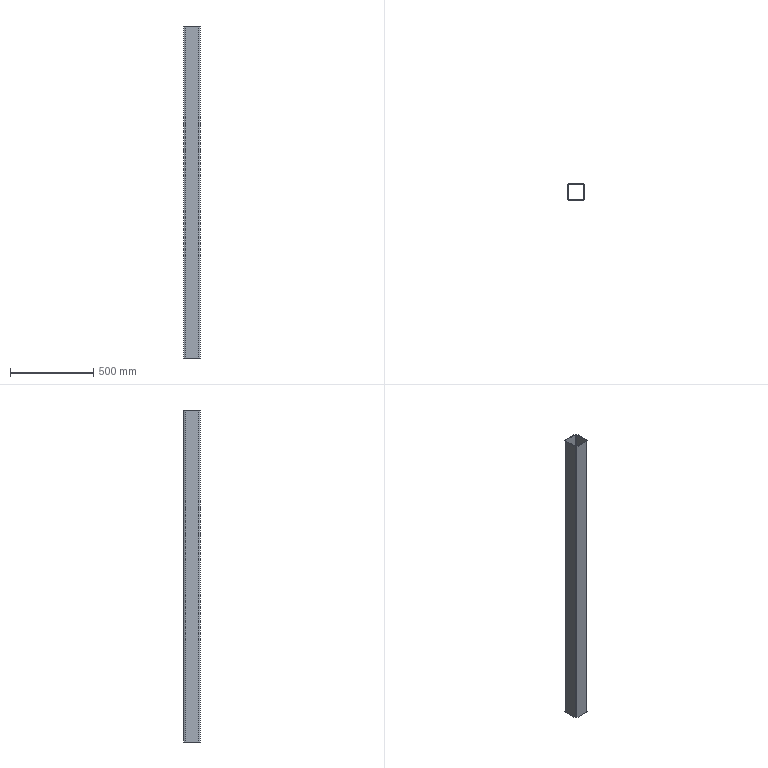Part | SolidWorks | features Extrusion 1, Fillet 1, HoleWzd 1, ICE 1, Shell 1 | 1 solid | 34 faces | box 100 x 100 x 2000 mm | volume 2980690 mm3 | cylinder 24 | plane 10 | commonest cylinder face diameters 6.8 x8 15 x8 8.8 x4 16.8 x4
STEP:
#1=CARTESIAN_POINT('',(-41.6,46.,1378.438));
#2=VERTEX_POINT('',#1);
#3=CARTESIAN_POINT('',(-35.,46.,1374.5));
#4=VERTEX_POINT('',#3);
#5=CARTESIAN_POINT('',(-35.,46.,1382.));
#6=DIRECTION('',(0.,-1.,0.));
#7=DIRECTION('',(0.,0.,-1.));
#8=AXIS2_PLACEMENT_3D('',#5,#6,#7);
#9=CIRCLE('',#8,7.5);
#10=EDGE_CURVE('',#2,#4,#9,.T.);
#11=ORIENTED_EDGE('',*,*,#10,.T.);
#12=CARTESIAN_POINT('',(-35.,50.,1374.5));
#13=VERTEX_POINT('',#12);
#14=CARTESIAN_POINT('',(-35.,40.,1374.5));
#15=DIRECTION('',(0.,1.,0.));
#16=VECTOR('',#15,1000.);
#17=LINE('',#14,#16);
#18=EDGE_CURVE('',#4,#13,#17,.T.);
#19=ORIENTED_EDGE('',*,*,#18,.T.);
#20=CARTESIAN_POINT('',(-41.6,50.,1378.438));
#21=VERTEX_POINT('',#20);
#22=CARTESIAN_POINT('',(-35.,50.,1382.));
#23=DIRECTION('',(0.,1.,0.));
#24=DIRECTION('',(0.,0.,1.));
#25=AXIS2_PLACEMENT_3D('',#22,#23,#24);
#26=CIRCLE('',#25,7.5);
#27=EDGE_CURVE('',#13,#21,#26,.T.);
#28=ORIENTED_EDGE('',*,*,#27,.T.);
#29=CARTESIAN_POINT('',(-41.6,50.,1385.562));
#30=VERTEX_POINT('',#29);
#31=CARTESIAN_POINT('',(-41.6,50.,1378.438));
#32=CARTESIAN_POINT('',(-41.897,50.,1378.987));
#33=CARTESIAN_POINT('',(-42.119,49.985,1379.562));
#34=CARTESIAN_POINT('',(-42.347,49.967,1380.459));
#35=CARTESIAN_POINT('',(-42.404,49.961,1380.767));
#36=CARTESIAN_POINT('',(-42.481,49.954,1381.383));
#37=CARTESIAN_POINT('',(-42.5,49.952,1381.691));
#38=CARTESIAN_POINT('',(-42.5,49.952,1382.307));
#39=CARTESIAN_POINT('',(-42.481,49.954,1382.614));
#40=CARTESIAN_POINT('',(-42.405,49.961,1383.229));
#41=CARTESIAN_POINT('',(-42.347,49.967,1383.537));
#42=CARTESIAN_POINT('',(-42.12,49.985,1384.438));
#43=CARTESIAN_POINT('',(-41.897,50.,1385.013));
#44=CARTESIAN_POINT('',(-41.6,50.,1385.562));
#45=B_SPLINE_CURVE_WITH_KNOTS('',3,(#31,#32,#33,#34,#35,#36,#37,#38,#39,#40,#41,#42,#43,#44),.UNSPECIFIED.,.F.,.F.,(4,2,2,2,2,2,4),(0.,0.001847,0.00277,0.003694,0.004617,0.00554,0.007387),.UNSPECIFIED.);
#46=EDGE_CURVE('',#21,#30,#45,.T.);
#47=ORIENTED_EDGE('',*,*,#46,.T.);
#48=CARTESIAN_POINT('',(-35.,50.,1389.5));
#49=VERTEX_POINT('',#48);
#50=CARTESIAN_POINT('',(-35.,50.,1382.));
#51=DIRECTION('',(0.,1.,0.));
#52=DIRECTION('',(0.,0.,1.));
#53=AXIS2_PLACEMENT_3D('',#50,#51,#52);
#54=CIRCLE('',#53,7.5);
#55=EDGE_CURVE('',#30,#49,#54,.T.);
#56=ORIENTED_EDGE('',*,*,#55,.T.);
#57=CARTESIAN_POINT('',(-35.,46.,1389.5));
#58=VERTEX_POINT('',#57);
#59=CARTESIAN_POINT('',(-35.,40.,1389.5));
#60=DIRECTION('',(0.,1.,0.));
#61=VECTOR('',#60,1000.);
#62=LINE('',#59,#61);
#63=EDGE_CURVE('',#58,#49,#62,.T.);
#64=ORIENTED_EDGE('',*,*,#63,.F.);
#65=CARTESIAN_POINT('',(-41.6,46.,1385.562));
#66=VERTEX_POINT('',#65);
#67=CARTESIAN_POINT('',(-35.,46.,1382.));
#68=DIRECTION('',(0.,-1.,0.));
#69=DIRECTION('',(0.,0.,-1.));
#70=AXIS2_PLACEMENT_3D('',#67,#68,#69);
#71=CIRCLE('',#70,7.5);
#72=EDGE_CURVE('',#58,#66,#71,.T.);
#73=ORIENTED_EDGE('',*,*,#72,.T.);
#74=CARTESIAN_POINT('',(-41.6,46.,1378.438));
#75=CARTESIAN_POINT('',(-41.897,46.,1378.988));
#76=CARTESIAN_POINT('',(-42.12,45.972,1379.563));
#77=CARTESIAN_POINT('',(-42.348,45.937,1380.466));
#78=CARTESIAN_POINT('',(-42.406,45.926,1380.774));
#79=CARTESIAN_POINT('',(-42.481,45.911,1381.387));
#80=CARTESIAN_POINT('',(-42.5,45.907,1381.695));
#81=CARTESIAN_POINT('',(-42.5,45.907,1382.311));
#82=CARTESIAN_POINT('',(-42.481,45.911,1382.619));
#83=CARTESIAN_POINT('',(-42.404,45.926,1383.238));
#84=CARTESIAN_POINT('',(-42.346,45.937,1383.543));
#85=CARTESIAN_POINT('',(-42.119,45.972,1384.439));
#86=CARTESIAN_POINT('',(-41.897,46.,1385.012));
#87=CARTESIAN_POINT('',(-41.6,46.,1385.562));
#88=B_SPLINE_CURVE_WITH_KNOTS('',3,(#74,#75,#76,#77,#78,#79,#80,#81,#82,#83,#84,#85,#86,#87),.UNSPECIFIED.,.F.,.F.,(4,2,2,2,2,2,4),(0.,0.001853,0.00278,0.003707,0.004633,0.00556,0.007413),.UNSPECIFIED.);
#89=EDGE_CURVE('',#2,#66,#88,.T.);
#90=ORIENTED_EDGE('',*,*,#89,.F.);
#91=EDGE_LOOP('',(#11,#19,#28,#47,#56,#64,#73,#90));
#92=FACE_OUTER_BOUND('',#91,.T.);
#93=CARTESIAN_POINT('',(-35.,40.,1382.));
#94=DIRECTION('',(0.,1.,0.));
#95=DIRECTION('',(0.,0.,1.));
#96=AXIS2_PLACEMENT_3D('',#93,#94,#95);
#97=CYLINDRICAL_SURFACE('',#96,7.5);
#98=ADVANCED_FACE('',(#92),#97,.F.);
#99=CARTESIAN_POINT('',(-41.6,46.,614.438));
#100=VERTEX_POINT('',#99);
#101=CARTESIAN_POINT('',(-35.,46.,610.5));
#102=VERTEX_POINT('',#101);
#103=CARTESIAN_POINT('',(-35.,46.,618.));
#104=DIRECTION('',(0.,-1.,0.));
#105=DIRECTION('',(0.,0.,-1.));
#106=AXIS2_PLACEMENT_3D('',#103,#104,#105);
#107=CIRCLE('',#106,7.5);
#108=EDGE_CURVE('',#100,#102,#107,.T.);
#109=ORIENTED_EDGE('',*,*,#108,.T.);
#110=CARTESIAN_POINT('',(-35.,50.,610.5));
#111=VERTEX_POINT('',#110);
#112=CARTESIAN_POINT('',(-35.,40.,610.5));
#113=DIRECTION('',(0.,1.,0.));
#114=VECTOR('',#113,1000.);
#115=LINE('',#112,#114);
#116=EDGE_CURVE('',#102,#111,#115,.T.);
#117=ORIENTED_EDGE('',*,*,#116,.T.);
#118=CARTESIAN_POINT('',(-41.6,50.,614.438));
#119=VERTEX_POINT('',#118);
#120=CARTESIAN_POINT('',(-35.,50.,618.));
#121=DIRECTION('',(0.,1.,0.));
#122=DIRECTION('',(0.,0.,1.));
#123=AXIS2_PLACEMENT_3D('',#120,#121,#122);
#124=CIRCLE('',#123,7.5);
#125=EDGE_CURVE('',#111,#119,#124,.T.);
#126=ORIENTED_EDGE('',*,*,#125,.T.);
#127=CARTESIAN_POINT('',(-41.6,50.,621.562));
#128=VERTEX_POINT('',#127);
#129=CARTESIAN_POINT('',(-41.6,50.,614.438));
#130=CARTESIAN_POINT('',(-41.897,50.,614.987));
#131=CARTESIAN_POINT('',(-42.119,49.985,615.562));
#132=CARTESIAN_POINT('',(-42.347,49.967,616.459));
#133=CARTESIAN_POINT('',(-42.404,49.961,616.767));
#134=CARTESIAN_POINT('',(-42.481,49.954,617.383));
#135=CARTESIAN_POINT('',(-42.5,49.952,617.691));
#136=CARTESIAN_POINT('',(-42.5,49.952,618.307));
#137=CARTESIAN_POINT('',(-42.481,49.954,618.614));
#138=CARTESIAN_POINT('',(-42.405,49.961,619.229));
#139=CARTESIAN_POINT('',(-42.347,49.967,619.537));
#140=CARTESIAN_POINT('',(-42.12,49.985,620.438));
#141=CARTESIAN_POINT('',(-41.897,50.,621.013));
#142=CARTESIAN_POINT('',(-41.6,50.,621.562));
#143=B_SPLINE_CURVE_WITH_KNOTS('',3,(#129,#130,#131,#132,#133,#134,#135,#136,#137,#138,#139,#140,#141,#142),.UNSPECIFIED.,.F.,.F.,(4,2,2,2,2,2,4),(0.,0.001847,0.00277,0.003694,0.004617,0.00554,0.007387),.UNSPECIFIED.);
#144=EDGE_CURVE('',#119,#128,#143,.T.);
#145=ORIENTED_EDGE('',*,*,#144,.T.);
#146=CARTESIAN_POINT('',(-35.,50.,625.5));
#147=VERTEX_POINT('',#146);
#148=CARTESIAN_POINT('',(-35.,50.,618.));
#149=DIRECTION('',(0.,1.,0.));
#150=DIRECTION('',(0.,0.,1.));
#151=AXIS2_PLACEMENT_3D('',#148,#149,#150);
#152=CIRCLE('',#151,7.5);
#153=EDGE_CURVE('',#128,#147,#152,.T.);
#154=ORIENTED_EDGE('',*,*,#153,.T.);
#155=CARTESIAN_POINT('',(-35.,46.,625.5));
#156=VERTEX_POINT('',#155);
#157=CARTESIAN_POINT('',(-35.,40.,625.5));
#158=DIRECTION('',(0.,1.,0.));
#159=VECTOR('',#158,1000.);
#160=LINE('',#157,#159);
#161=EDGE_CURVE('',#156,#147,#160,.T.);
#162=ORIENTED_EDGE('',*,*,#161,.F.);
#163=CARTESIAN_POINT('',(-41.6,46.,621.562));
#164=VERTEX_POINT('',#163);
#165=CARTESIAN_POINT('',(-35.,46.,618.));
#166=DIRECTION('',(0.,-1.,0.));
#167=DIRECTION('',(0.,0.,-1.));
#168=AXIS2_PLACEMENT_3D('',#165,#166,#167);
#169=CIRCLE('',#168,7.5);
#170=EDGE_CURVE('',#156,#164,#169,.T.);
#171=ORIENTED_EDGE('',*,*,#170,.T.);
#172=CARTESIAN_POINT('',(-41.6,46.,614.438));
#173=CARTESIAN_POINT('',(-41.897,46.,614.988));
#174=CARTESIAN_POINT('',(-42.12,45.972,615.563));
#175=CARTESIAN_POINT('',(-42.348,45.937,616.466));
#176=CARTESIAN_POINT('',(-42.406,45.926,616.774));
#177=CARTESIAN_POINT('',(-42.481,45.911,617.387));
#178=CARTESIAN_POINT('',(-42.5,45.907,617.695));
#179=CARTESIAN_POINT('',(-42.5,45.907,618.311));
#180=CARTESIAN_POINT('',(-42.481,45.911,618.619));
#181=CARTESIAN_POINT('',(-42.404,45.926,619.238));
#182=CARTESIAN_POINT('',(-42.346,45.937,619.543));
#183=CARTESIAN_POINT('',(-42.119,45.972,620.439));
#184=CARTESIAN_POINT('',(-41.897,46.,621.012));
#185=CARTESIAN_POINT('',(-41.6,46.,621.562));
#186=B_SPLINE_CURVE_WITH_KNOTS('',3,(#172,#173,#174,#175,#176,#177,#178,#179,#180,#181,#182,#183,#184,#185),.UNSPECIFIED.,.F.,.F.,(4,2,2,2,2,2,4),(0.,0.001853,0.00278,0.003707,0.004633,0.00556,0.007413),.UNSPECIFIED.);
#187=EDGE_CURVE('',#100,#164,#186,.T.);
#188=ORIENTED_EDGE('',*,*,#187,.F.);
#189=EDGE_LOOP('',(#109,#117,#126,#145,#154,#162,#171,#188));
#190=FACE_OUTER_BOUND('',#189,.T.);
#191=CARTESIAN_POINT('',(-35.,40.,618.));
#192=DIRECTION('',(0.,1.,0.));
#193=DIRECTION('',(0.,0.,1.));
#194=AXIS2_PLACEMENT_3D('',#191,#192,#193);
#195=CYLINDRICAL_SURFACE('',#194,7.5);
#196=ADVANCED_FACE('',(#190),#195,.F.);
#197=CARTESIAN_POINT('',(35.,46.,1389.5));
#198=VERTEX_POINT('',#197);
#199=CARTESIAN_POINT('',(35.,46.,1374.5));
#200=VERTEX_POINT('',#199);
#201=CARTESIAN_POINT('',(35.,46.,1382.));
#202=DIRECTION('',(0.,-1.,0.));
#203=DIRECTION('',(0.,0.,-1.));
#204=AXIS2_PLACEMENT_3D('',#201,#202,#203);
#205=CIRCLE('',#204,7.5);
#206=EDGE_CURVE('',#198,#200,#205,.T.);
#207=ORIENTED_EDGE('',*,*,#206,.T.);
#208=CARTESIAN_POINT('',(35.,50.,1374.5));
#209=VERTEX_POINT('',#208);
#210=CARTESIAN_POINT('',(35.,40.,1374.5));
#211=DIRECTION('',(0.,1.,0.));
#212=VECTOR('',#211,1000.);
#213=LINE('',#210,#212);
#214=EDGE_CURVE('',#200,#209,#213,.T.);
#215=ORIENTED_EDGE('',*,*,#214,.T.);
#216=CARTESIAN_POINT('',(35.,50.,1389.5));
#217=VERTEX_POINT('',#216);
#218=CARTESIAN_POINT('',(35.,50.,1382.));
#219=DIRECTION('',(0.,1.,0.));
#220=DIRECTION('',(0.,0.,1.));
#221=AXIS2_PLACEMENT_3D('',#218,#219,#220);
#222=CIRCLE('',#221,7.5);
#223=EDGE_CURVE('',#209,#217,#222,.T.);
#224=ORIENTED_EDGE('',*,*,#223,.T.);
#225=CARTESIAN_POINT('',(35.,40.,1389.5));
#226=DIRECTION('',(0.,1.,0.));
#227=VECTOR('',#226,1000.);
#228=LINE('',#225,#227);
#229=EDGE_CURVE('',#198,#217,#228,.T.);
#230=ORIENTED_EDGE('',*,*,#229,.F.);
#231=EDGE_LOOP('',(#207,#215,#224,#230));
#232=FACE_OUTER_BOUND('',#231,.T.);
#233=CARTESIAN_POINT('',(35.,40.,1382.));
#234=DIRECTION('',(0.,1.,0.));
#235=DIRECTION('',(0.,0.,1.));
#236=AXIS2_PLACEMENT_3D('',#233,#234,#235);
#237=CYLINDRICAL_SURFACE('',#236,7.5);
#238=ADVANCED_FACE('',(#232),#237,.F.);
#239=CARTESIAN_POINT('',(35.,46.,625.5));
#240=VERTEX_POINT('',#239);
#241=CARTESIAN_POINT('',(35.,46.,610.5));
#242=VERTEX_POINT('',#241);
#243=CARTESIAN_POINT('',(35.,46.,618.));
#244=DIRECTION('',(0.,-1.,0.));
#245=DIRECTION('',(0.,0.,-1.));
#246=AXIS2_PLACEMENT_3D('',#243,#244,#245);
#247=CIRCLE('',#246,7.5);
#248=EDGE_CURVE('',#240,#242,#247,.T.);
#249=ORIENTED_EDGE('',*,*,#248,.T.);
#250=CARTESIAN_POINT('',(35.,50.,610.5));
#251=VERTEX_POINT('',#250);
#252=CARTESIAN_POINT('',(35.,40.,610.5));
#253=DIRECTION('',(0.,1.,0.));
#254=VECTOR('',#253,1000.);
#255=LINE('',#252,#254);
#256=EDGE_CURVE('',#242,#251,#255,.T.);
#257=ORIENTED_EDGE('',*,*,#256,.T.);
#258=CARTESIAN_POINT('',(35.,50.,625.5));
#259=VERTEX_POINT('',#258);
#260=CARTESIAN_POINT('',(35.,50.,618.));
#261=DIRECTION('',(0.,1.,0.));
#262=DIRECTION('',(0.,0.,1.));
#263=AXIS2_PLACEMENT_3D('',#260,#261,#262);
#264=CIRCLE('',#263,7.5);
#265=EDGE_CURVE('',#251,#259,#264,.T.);
#266=ORIENTED_EDGE('',*,*,#265,.T.);
#267=CARTESIAN_POINT('',(35.,40.,625.5));
#268=DIRECTION('',(0.,1.,0.));
#269=VECTOR('',#268,1000.);
#270=LINE('',#267,#269);
#271=EDGE_CURVE('',#240,#259,#270,.T.);
#272=ORIENTED_EDGE('',*,*,#271,.F.);
#273=EDGE_LOOP('',(#249,#257,#266,#272));
#274=FACE_OUTER_BOUND('',#273,.T.);
#275=CARTESIAN_POINT('',(35.,40.,618.));
#276=DIRECTION('',(0.,1.,0.));
#277=DIRECTION('',(0.,0.,1.));
#278=AXIS2_PLACEMENT_3D('',#275,#276,#277);
#279=CYLINDRICAL_SURFACE('',#278,7.5);
#280=ADVANCED_FACE('',(#274),#279,.F.);
#281=CARTESIAN_POINT('',(-35.,46.,393.4));
#282=VERTEX_POINT('',#281);
#283=CARTESIAN_POINT('',(-35.,46.,386.6));
#284=VERTEX_POINT('',#283);
#285=CARTESIAN_POINT('',(-35.,46.,390.));
#286=DIRECTION('',(0.,-1.,0.));
#287=DIRECTION('',(0.,0.,-1.));
#288=AXIS2_PLACEMENT_3D('',#285,#286,#287);
#289=CIRCLE('',#288,3.4);
#290=EDGE_CURVE('',#282,#284,#289,.T.);
#291=ORIENTED_EDGE('',*,*,#290,.T.);
#292=CARTESIAN_POINT('',(-35.,50.,386.6));
#293=VERTEX_POINT('',#292);
#294=CARTESIAN_POINT('',(-35.,50.,386.6));
#295=DIRECTION('',(0.,1.,0.));
#296=VECTOR('',#295,1000.);
#297=LINE('',#294,#296);
#298=EDGE_CURVE('',#284,#293,#297,.T.);
#299=ORIENTED_EDGE('',*,*,#298,.T.);
#300=CARTESIAN_POINT('',(-35.,50.,393.4));
#301=VERTEX_POINT('',#300);
#302=CARTESIAN_POINT('',(-35.,50.,390.));
#303=DIRECTION('',(0.,1.,0.));
#304=DIRECTION('',(0.,0.,1.));
#305=AXIS2_PLACEMENT_3D('',#302,#303,#304);
#306=CIRCLE('',#305,3.4);
#307=EDGE_CURVE('',#293,#301,#306,.T.);
#308=ORIENTED_EDGE('',*,*,#307,.T.);
#309=CARTESIAN_POINT('',(-35.,50.,393.4));
#310=DIRECTION('',(0.,1.,0.));
#311=VECTOR('',#310,1000.);
#312=LINE('',#309,#311);
#313=EDGE_CURVE('',#282,#301,#312,.T.);
#314=ORIENTED_EDGE('',*,*,#313,.F.);
#315=EDGE_LOOP('',(#291,#299,#308,#314));
#316=FACE_OUTER_BOUND('',#315,.T.);
#317=CARTESIAN_POINT('',(-35.,50.,390.));
#318=DIRECTION('',(0.,1.,0.));
#319=DIRECTION('',(0.,0.,1.));
#320=AXIS2_PLACEMENT_3D('',#317,#318,#319);
#321=CYLINDRICAL_SURFACE('',#320,3.4);
#322=ADVANCED_FACE('',(#316),#321,.F.);
#323=CARTESIAN_POINT('',(35.,46.,393.4));
#324=VERTEX_POINT('',#323);
#325=CARTESIAN_POINT('',(35.,46.,386.6));
#326=VERTEX_POINT('',#325);
#327=CARTESIAN_POINT('',(35.,46.,390.));
#328=DIRECTION('',(0.,-1.,0.));
#329=DIRECTION('',(0.,0.,-1.));
#330=AXIS2_PLACEMENT_3D('',#327,#328,#329);
#331=CIRCLE('',#330,3.4);
#332=EDGE_CURVE('',#324,#326,#331,.T.);
#333=ORIENTED_EDGE('',*,*,#332,.T.);
#334=CARTESIAN_POINT('',(35.,50.,386.6));
#335=VERTEX_POINT('',#334);
#336=CARTESIAN_POINT('',(35.,50.,386.6));
#337=DIRECTION('',(0.,1.,0.));
#338=VECTOR('',#337,1000.);
#339=LINE('',#336,#338);
#340=EDGE_CURVE('',#326,#335,#339,.T.);
#341=ORIENTED_EDGE('',*,*,#340,.T.);
#342=CARTESIAN_POINT('',(35.,50.,393.4));
#343=VERTEX_POINT('',#342);
#344=CARTESIAN_POINT('',(35.,50.,390.));
#345=DIRECTION('',(0.,1.,0.));
#346=DIRECTION('',(0.,0.,1.));
#347=AXIS2_PLACEMENT_3D('',#344,#345,#346);
#348=CIRCLE('',#347,3.4);
#349=EDGE_CURVE('',#335,#343,#348,.T.);
#350=ORIENTED_EDGE('',*,*,#349,.T.);
#351=CARTESIAN_POINT('',(35.,50.,393.4));
#352=DIRECTION('',(0.,1.,0.));
#353=VECTOR('',#352,1000.);
#354=LINE('',#351,#353);
#355=EDGE_CURVE('',#324,#343,#354,.T.);
#356=ORIENTED_EDGE('',*,*,#355,.F.);
#357=EDGE_LOOP('',(#333,#341,#350,#356));
#358=FACE_OUTER_BOUND('',#357,.T.);
#359=CARTESIAN_POINT('',(35.,50.,390.));
#360=DIRECTION('',(0.,1.,0.));
#361=DIRECTION('',(0.,0.,1.));
#362=AXIS2_PLACEMENT_3D('',#359,#360,#361);
#363=CYLINDRICAL_SURFACE('',#362,3.4);
#364=ADVANCED_FACE('',(#358),#363,.F.);
#365=CARTESIAN_POINT('',(35.,46.,483.4));
#366=VERTEX_POINT('',#365);
#367=CARTESIAN_POINT('',(35.,46.,476.6));
#368=VERTEX_POINT('',#367);
#369=CARTESIAN_POINT('',(35.,46.,480.));
#370=DIRECTION('',(0.,-1.,0.));
#371=DIRECTION('',(0.,0.,-1.));
#372=AXIS2_PLACEMENT_3D('',#369,#370,#371);
#373=CIRCLE('',#372,3.4);
#374=EDGE_CURVE('',#366,#368,#373,.T.);
#375=ORIENTED_EDGE('',*,*,#374,.T.);
#376=CARTESIAN_POINT('',(35.,50.,476.6));
#377=VERTEX_POINT('',#376);
#378=CARTESIAN_POINT('',(35.,50.,476.6));
#379=DIRECTION('',(0.,1.,0.));
#380=VECTOR('',#379,1000.);
#381=LINE('',#378,#380);
#382=EDGE_CURVE('',#368,#377,#381,.T.);
#383=ORIENTED_EDGE('',*,*,#382,.T.);
#384=CARTESIAN_POINT('',(35.,50.,483.4));
#385=VERTEX_POINT('',#384);
#386=CARTESIAN_POINT('',(35.,50.,480.));
#387=DIRECTION('',(0.,1.,0.));
#388=DIRECTION('',(0.,0.,1.));
#389=AXIS2_PLACEMENT_3D('',#386,#387,#388);
#390=CIRCLE('',#389,3.4);
#391=EDGE_CURVE('',#377,#385,#390,.T.);
#392=ORIENTED_EDGE('',*,*,#391,.T.);
#393=CARTESIAN_POINT('',(35.,50.,483.4));
#394=DIRECTION('',(0.,1.,0.));
#395=VECTOR('',#394,1000.);
#396=LINE('',#393,#395);
#397=EDGE_CURVE('',#366,#385,#396,.T.);
#398=ORIENTED_EDGE('',*,*,#397,.F.);
#399=EDGE_LOOP('',(#375,#383,#392,#398));
#400=FACE_OUTER_BOUND('',#399,.T.);
#401=CARTESIAN_POINT('',(35.,50.,480.));
#402=DIRECTION('',(0.,1.,0.));
#403=DIRECTION('',(0.,0.,1.));
#404=AXIS2_PLACEMENT_3D('',#401,#402,#403);
#405=CYLINDRICAL_SURFACE('',#404,3.4);
#406=ADVANCED_FACE('',(#400),#405,.F.);
#407=CARTESIAN_POINT('',(-35.,46.,483.4));
#408=VERTEX_POINT('',#407);
#409=CARTESIAN_POINT('',(-35.,46.,476.6));
#410=VERTEX_POINT('',#409);
#411=CARTESIAN_POINT('',(-35.,46.,480.));
#412=DIRECTION('',(0.,-1.,0.));
#413=DIRECTION('',(0.,0.,-1.));
#414=AXIS2_PLACEMENT_3D('',#411,#412,#413);
#415=CIRCLE('',#414,3.4);
#416=EDGE_CURVE('',#408,#410,#415,.T.);
#417=ORIENTED_EDGE('',*,*,#416,.T.);
#418=CARTESIAN_POINT('',(-35.,50.,476.6));
#419=VERTEX_POINT('',#418);
#420=CARTESIAN_POINT('',(-35.,50.,476.6));
#421=DIRECTION('',(0.,1.,0.));
#422=VECTOR('',#421,1000.);
#423=LINE('',#420,#422);
#424=EDGE_CURVE('',#410,#419,#423,.T.);
#425=ORIENTED_EDGE('',*,*,#424,.T.);
#426=CARTESIAN_POINT('',(-35.,50.,483.4));
#427=VERTEX_POINT('',#426);
#428=CARTESIAN_POINT('',(-35.,50.,480.));
#429=DIRECTION('',(0.,1.,0.));
#430=DIRECTION('',(0.,0.,1.));
#431=AXIS2_PLACEMENT_3D('',#428,#429,#430);
#432=CIRCLE('',#431,3.4);
#433=EDGE_CURVE('',#419,#427,#432,.T.);
#434=ORIENTED_EDGE('',*,*,#433,.T.);
#435=CARTESIAN_POINT('',(-35.,50.,483.4));
#436=DIRECTION('',(0.,1.,0.));
#437=VECTOR('',#436,1000.);
#438=LINE('',#435,#437);
#439=EDGE_CURVE('',#408,#427,#438,.T.);
#440=ORIENTED_EDGE('',*,*,#439,.F.);
#441=EDGE_LOOP('',(#417,#425,#434,#440));
#442=FACE_OUTER_BOUND('',#441,.T.);
#443=CARTESIAN_POINT('',(-35.,50.,480.));
#444=DIRECTION('',(0.,1.,0.));
#445=DIRECTION('',(0.,0.,1.));
#446=AXIS2_PLACEMENT_3D('',#443,#444,#445);
#447=CYLINDRICAL_SURFACE('',#446,3.4);
#448=ADVANCED_FACE('',(#442),#447,.F.);
#449=CARTESIAN_POINT('',(50.,-41.6,0.));
#450=VERTEX_POINT('',#449);
#451=CARTESIAN_POINT('',(50.,41.6,0.));
#452=VERTEX_POINT('',#451);
#453=CARTESIAN_POINT('',(50.,50.,0.));
#454=DIRECTION('',(0.,1.,0.));
#455=VECTOR('',#454,1000.);
#456=LINE('',#453,#455);
#457=EDGE_CURVE('',#450,#452,#456,.T.);
#458=ORIENTED_EDGE('',*,*,#457,.F.);
#459=CARTESIAN_POINT('',(41.6,-50.,0.));
#460=VERTEX_POINT('',#459);
#461=CARTESIAN_POINT('',(41.6,-41.6,0.));
#462=DIRECTION('',(0.,0.,-1.));
#463=DIRECTION('',(-1.,0.,0.));
#464=AXIS2_PLACEMENT_3D('',#461,#462,#463);
#465=CIRCLE('',#464,8.4);
#466=EDGE_CURVE('',#450,#460,#465,.T.);
#467=ORIENTED_EDGE('',*,*,#466,.T.);
#468=CARTESIAN_POINT('',(-41.6,-50.,0.));
#469=VERTEX_POINT('',#468);
#470=CARTESIAN_POINT('',(50.,-50.,0.));
#471=DIRECTION('',(1.,0.,0.));
#472=VECTOR('',#471,1000.);
#473=LINE('',#470,#472);
#474=EDGE_CURVE('',#469,#460,#473,.T.);
#475=ORIENTED_EDGE('',*,*,#474,.F.);
#476=CARTESIAN_POINT('',(-50.,-41.6,0.));
#477=VERTEX_POINT('',#476);
#478=CARTESIAN_POINT('',(-41.6,-41.6,0.));
#479=DIRECTION('',(0.,0.,-1.));
#480=DIRECTION('',(-1.,0.,0.));
#481=AXIS2_PLACEMENT_3D('',#478,#479,#480);
#482=CIRCLE('',#481,8.4);
#483=EDGE_CURVE('',#469,#477,#482,.T.);
#484=ORIENTED_EDGE('',*,*,#483,.T.);
#485=CARTESIAN_POINT('',(-50.,41.6,0.));
#486=VERTEX_POINT('',#485);
#487=CARTESIAN_POINT('',(-50.,50.,0.));
#488=DIRECTION('',(0.,-1.,0.));
#489=VECTOR('',#488,1000.);
#490=LINE('',#487,#489);
#491=EDGE_CURVE('',#486,#477,#490,.T.);
#492=ORIENTED_EDGE('',*,*,#491,.F.);
#493=CARTESIAN_POINT('',(-41.6,50.,0.));
#494=VERTEX_POINT('',#493);
#495=CARTESIAN_POINT('',(-41.6,41.6,0.));
#496=DIRECTION('',(0.,0.,-1.));
#497=DIRECTION('',(-1.,0.,0.));
#498=AXIS2_PLACEMENT_3D('',#495,#496,#497);
#499=CIRCLE('',#498,8.4);
#500=EDGE_CURVE('',#486,#494,#499,.T.);
#501=ORIENTED_EDGE('',*,*,#500,.T.);
#502=CARTESIAN_POINT('',(41.6,50.,0.));
#503=VERTEX_POINT('',#502);
#504=CARTESIAN_POINT('',(50.,50.,0.));
#505=DIRECTION('',(-1.,0.,0.));
#506=VECTOR('',#505,1000.);
#507=LINE('',#504,#506);
#508=EDGE_CURVE('',#503,#494,#507,.T.);
#509=ORIENTED_EDGE('',*,*,#508,.F.);
#510=CARTESIAN_POINT('',(41.6,41.6,0.));
#511=DIRECTION('',(0.,0.,-1.));
#512=DIRECTION('',(-1.,0.,0.));
#513=AXIS2_PLACEMENT_3D('',#510,#511,#512);
#514=CIRCLE('',#513,8.4);
#515=EDGE_CURVE('',#503,#452,#514,.T.);
#516=ORIENTED_EDGE('',*,*,#515,.T.);
#517=EDGE_LOOP('',(#458,#467,#475,#484,#492,#501,#509,#516));
#518=FACE_OUTER_BOUND('',#517,.T.);
#519=CARTESIAN_POINT('',(46.,-41.6,0.));
#520=VERTEX_POINT('',#519);
#521=CARTESIAN_POINT('',(41.6,-46.,0.));
#522=VERTEX_POINT('',#521);
#523=CARTESIAN_POINT('',(41.6,-41.6,0.));
#524=DIRECTION('',(0.,0.,-1.));
#525=DIRECTION('',(-1.,0.,0.));
#526=AXIS2_PLACEMENT_3D('',#523,#524,#525);
#527=CIRCLE('',#526,4.4);
#528=EDGE_CURVE('',#520,#522,#527,.T.);
#529=ORIENTED_EDGE('',*,*,#528,.F.);
#530=CARTESIAN_POINT('',(46.,41.6,0.));
#531=VERTEX_POINT('',#530);
#532=CARTESIAN_POINT('',(46.,0.,0.));
#533=DIRECTION('',(0.,1.,0.));
#534=VECTOR('',#533,1000.);
#535=LINE('',#532,#534);
#536=EDGE_CURVE('',#520,#531,#535,.T.);
#537=ORIENTED_EDGE('',*,*,#536,.T.);
#538=CARTESIAN_POINT('',(41.6,46.,0.));
#539=VERTEX_POINT('',#538);
#540=CARTESIAN_POINT('',(41.6,41.6,0.));
#541=DIRECTION('',(0.,0.,-1.));
#542=DIRECTION('',(-1.,0.,0.));
#543=AXIS2_PLACEMENT_3D('',#540,#541,#542);
#544=CIRCLE('',#543,4.4);
#545=EDGE_CURVE('',#539,#531,#544,.T.);
#546=ORIENTED_EDGE('',*,*,#545,.F.);
#547=CARTESIAN_POINT('',(-41.6,46.,0.));
#548=VERTEX_POINT('',#547);
#549=CARTESIAN_POINT('',(0.,46.,0.));
#550=DIRECTION('',(-1.,0.,0.));
#551=VECTOR('',#550,1000.);
#552=LINE('',#549,#551);
#553=EDGE_CURVE('',#539,#548,#552,.T.);
#554=ORIENTED_EDGE('',*,*,#553,.T.);
#555=CARTESIAN_POINT('',(-46.,41.6,0.));
#556=VERTEX_POINT('',#555);
#557=CARTESIAN_POINT('',(-41.6,41.6,0.));
#558=DIRECTION('',(0.,0.,-1.));
#559=DIRECTION('',(-1.,0.,0.));
#560=AXIS2_PLACEMENT_3D('',#557,#558,#559);
#561=CIRCLE('',#560,4.4);
#562=EDGE_CURVE('',#556,#548,#561,.T.);
#563=ORIENTED_EDGE('',*,*,#562,.F.);
#564=CARTESIAN_POINT('',(-46.,-41.6,0.));
#565=VERTEX_POINT('',#564);
#566=CARTESIAN_POINT('',(-46.,0.,0.));
#567=DIRECTION('',(0.,-1.,0.));
#568=VECTOR('',#567,1000.);
#569=LINE('',#566,#568);
#570=EDGE_CURVE('',#556,#565,#569,.T.);
#571=ORIENTED_EDGE('',*,*,#570,.T.);
#572=CARTESIAN_POINT('',(-41.6,-46.,0.));
#573=VERTEX_POINT('',#572);
#574=CARTESIAN_POINT('',(-41.6,-41.6,0.));
#575=DIRECTION('',(0.,0.,-1.));
#576=DIRECTION('',(-1.,0.,0.));
#577=AXIS2_PLACEMENT_3D('',#574,#575,#576);
#578=CIRCLE('',#577,4.4);
#579=EDGE_CURVE('',#573,#565,#578,.T.);
#580=ORIENTED_EDGE('',*,*,#579,.F.);
#581=CARTESIAN_POINT('',(0.,-46.,0.));
#582=DIRECTION('',(1.,0.,0.));
#583=VECTOR('',#582,1000.);
#584=LINE('',#581,#583);
#585=EDGE_CURVE('',#573,#522,#584,.T.);
#586=ORIENTED_EDGE('',*,*,#585,.T.);
#587=EDGE_LOOP('',(#529,#537,#546,#554,#563,#571,#580,#586));
#588=FACE_BOUND('',#587,.T.);
#589=CARTESIAN_POINT('',(0.,0.,0.));
#590=DIRECTION('',(0.,0.,-1.));
#591=DIRECTION('',(-1.,0.,0.));
#592=AXIS2_PLACEMENT_3D('',#589,#590,#591);
#593=PLANE('',#592);
#594=ADVANCED_FACE('',(#518,#588),#593,.T.);
#595=ORIENTED_EDGE('',*,*,#491,.T.);
#596=CARTESIAN_POINT('',(-50.,-41.6,2000.));
#597=VERTEX_POINT('',#596);
#598=CARTESIAN_POINT('',(-50.,-41.6,2000.));
#599=DIRECTION('',(0.,0.,1.));
#600=VECTOR('',#599,1000.);
#601=LINE('',#598,#600);
#602=EDGE_CURVE('',#477,#597,#601,.T.);
#603=ORIENTED_EDGE('',*,*,#602,.T.);
#604=CARTESIAN_POINT('',(-50.,41.6,2000.));
#605=VERTEX_POINT('',#604);
#606=CARTESIAN_POINT('',(-50.,50.,2000.));
#607=DIRECTION('',(0.,-1.,0.));
#608=VECTOR('',#607,1000.);
#609=LINE('',#606,#608);
#610=EDGE_CURVE('',#605,#597,#609,.T.);
#611=ORIENTED_EDGE('',*,*,#610,.F.);
#612=CARTESIAN_POINT('',(-50.,41.6,2000.));
#613=DIRECTION('',(0.,0.,-1.));
#614=VECTOR('',#613,1000.);
#615=LINE('',#612,#614);
#616=EDGE_CURVE('',#605,#486,#615,.T.);
#617=ORIENTED_EDGE('',*,*,#616,.T.);
#618=EDGE_LOOP('',(#595,#603,#611,#617));
#619=FACE_OUTER_BOUND('',#618,.T.);
#620=CARTESIAN_POINT('',(-50.,50.,2000.));
#621=DIRECTION('',(1.,0.,0.));
#622=DIRECTION('',(0.,1.,0.));
#623=AXIS2_PLACEMENT_3D('',#620,#621,#622);
#624=PLANE('',#623);
#625=ADVANCED_FACE('',(#619),#624,.F.);
#626=ORIENTED_EDGE('',*,*,#474,.T.);
#627=CARTESIAN_POINT('',(41.6,-50.,2000.));
#628=VERTEX_POINT('',#627);
#629=CARTESIAN_POINT('',(41.6,-50.,2000.));
#630=DIRECTION('',(0.,0.,1.));
#631=VECTOR('',#630,1000.);
#632=LINE('',#629,#631);
#633=EDGE_CURVE('',#460,#628,#632,.T.);
#634=ORIENTED_EDGE('',*,*,#633,.T.);
#635=CARTESIAN_POINT('',(-41.6,-50.,2000.));
#636=VERTEX_POINT('',#635);
#637=CARTESIAN_POINT('',(50.,-50.,2000.));
#638=DIRECTION('',(1.,0.,0.));
#639=VECTOR('',#638,1000.);
#640=LINE('',#637,#639);
#641=EDGE_CURVE('',#636,#628,#640,.T.);
#642=ORIENTED_EDGE('',*,*,#641,.F.);
#643=CARTESIAN_POINT('',(-41.6,-50.,2000.));
#644=DIRECTION('',(0.,0.,-1.));
#645=VECTOR('',#644,1000.);
#646=LINE('',#643,#645);
#647=EDGE_CURVE('',#636,#469,#646,.T.);
#648=ORIENTED_EDGE('',*,*,#647,.T.);
#649=EDGE_LOOP('',(#626,#634,#642,#648));
#650=FACE_OUTER_BOUND('',#649,.T.);
#651=CARTESIAN_POINT('',(50.,-50.,2000.));
#652=DIRECTION('',(0.,1.,0.));
#653=DIRECTION('',(0.,0.,1.));
#654=AXIS2_PLACEMENT_3D('',#651,#652,#653);
#655=PLANE('',#654);
#656=ADVANCED_FACE('',(#650),#655,.F.);
#657=CARTESIAN_POINT('',(50.,-41.6,2000.));
#658=VERTEX_POINT('',#657);
#659=CARTESIAN_POINT('',(50.,41.6,2000.));
#660=VERTEX_POINT('',#659);
#661=CARTESIAN_POINT('',(50.,50.,2000.));
#662=DIRECTION('',(0.,1.,0.));
#663=VECTOR('',#662,1000.);
#664=LINE('',#661,#663);
#665=EDGE_CURVE('',#658,#660,#664,.T.);
#666=ORIENTED_EDGE('',*,*,#665,.F.);
#667=CARTESIAN_POINT('',(50.,-41.6,2000.));
#668=DIRECTION('',(0.,0.,-1.));
#669=VECTOR('',#668,1000.);
#670=LINE('',#667,#669);
#671=EDGE_CURVE('',#658,#450,#670,.T.);
#672=ORIENTED_EDGE('',*,*,#671,.T.);
#673=ORIENTED_EDGE('',*,*,#457,.T.);
#674=CARTESIAN_POINT('',(50.,41.6,2000.));
#675=DIRECTION('',(0.,0.,1.));
#676=VECTOR('',#675,1000.);
#677=LINE('',#674,#676);
#678=EDGE_CURVE('',#452,#660,#677,.T.);
#679=ORIENTED_EDGE('',*,*,#678,.T.);
#680=EDGE_LOOP('',(#666,#672,#673,#679));
#681=FACE_OUTER_BOUND('',#680,.T.);
#682=CARTESIAN_POINT('',(50.,50.,2000.));
#683=DIRECTION('',(-1.,0.,0.));
#684=DIRECTION('',(0.,-1.,0.));
#685=AXIS2_PLACEMENT_3D('',#682,#683,#684);
#686=PLANE('',#685);
#687=ADVANCED_FACE('',(#681),#686,.F.);
#688=CARTESIAN_POINT('',(-35.,50.,390.));
#689=DIRECTION('',(0.,1.,0.));
#690=DIRECTION('',(0.,0.,1.));
#691=AXIS2_PLACEMENT_3D('',#688,#689,#690);
#692=CIRCLE('',#691,3.4);
#693=EDGE_CURVE('',#301,#293,#692,.T.);
#694=ORIENTED_EDGE('',*,*,#693,.F.);
#695=ORIENTED_EDGE('',*,*,#307,.F.);
#696=EDGE_LOOP('',(#694,#695));
#697=FACE_BOUND('',#696,.T.);
#698=CARTESIAN_POINT('',(35.,50.,390.));
#699=DIRECTION('',(0.,1.,0.));
#700=DIRECTION('',(0.,0.,1.));
#701=AXIS2_PLACEMENT_3D('',#698,#699,#700);
#702=CIRCLE('',#701,3.4);
#703=EDGE_CURVE('',#343,#335,#702,.T.);
#704=ORIENTED_EDGE('',*,*,#703,.F.);
#705=ORIENTED_EDGE('',*,*,#349,.F.);
#706=EDGE_LOOP('',(#704,#705));
#707=FACE_BOUND('',#706,.T.);
#708=CARTESIAN_POINT('',(35.,50.,480.));
#709=DIRECTION('',(0.,1.,0.));
#710=DIRECTION('',(0.,0.,1.));
#711=AXIS2_PLACEMENT_3D('',#708,#709,#710);
#712=CIRCLE('',#711,3.4);
#713=EDGE_CURVE('',#385,#377,#712,.T.);
#714=ORIENTED_EDGE('',*,*,#713,.F.);
#715=ORIENTED_EDGE('',*,*,#391,.F.);
#716=EDGE_LOOP('',(#714,#715));
#717=FACE_BOUND('',#716,.T.);
#718=CARTESIAN_POINT('',(-35.,50.,480.));
#719=DIRECTION('',(0.,1.,0.));
#720=DIRECTION('',(0.,0.,1.));
#721=AXIS2_PLACEMENT_3D('',#718,#719,#720);
#722=CIRCLE('',#721,3.4);
#723=EDGE_CURVE('',#427,#419,#722,.T.);
#724=ORIENTED_EDGE('',*,*,#723,.F.);
#725=ORIENTED_EDGE('',*,*,#433,.F.);
#726=EDGE_LOOP('',(#724,#725));
#727=FACE_BOUND('',#726,.T.);
#728=CARTESIAN_POINT('',(-41.6,50.,2000.));
#729=DIRECTION('',(0.,0.,1.));
#730=VECTOR('',#729,1000.);
#731=LINE('',#728,#730);
#732=EDGE_CURVE('',#128,#21,#731,.T.);
#733=ORIENTED_EDGE('',*,*,#732,.T.);
#734=ORIENTED_EDGE('',*,*,#27,.F.);
#735=CARTESIAN_POINT('',(-35.,50.,1382.));
#736=DIRECTION('',(0.,1.,0.));
#737=DIRECTION('',(0.,0.,1.));
#738=AXIS2_PLACEMENT_3D('',#735,#736,#737);
#739=CIRCLE('',#738,7.5);
#740=EDGE_CURVE('',#49,#13,#739,.T.);
#741=ORIENTED_EDGE('',*,*,#740,.F.);
#742=ORIENTED_EDGE('',*,*,#55,.F.);
#743=CARTESIAN_POINT('',(-41.6,50.,2000.));
#744=VERTEX_POINT('',#743);
#745=CARTESIAN_POINT('',(-41.6,50.,2000.));
#746=DIRECTION('',(0.,0.,1.));
#747=VECTOR('',#746,1000.);
#748=LINE('',#745,#747);
#749=EDGE_CURVE('',#30,#744,#748,.T.);
#750=ORIENTED_EDGE('',*,*,#749,.T.);
#751=CARTESIAN_POINT('',(41.6,50.,2000.));
#752=VERTEX_POINT('',#751);
#753=CARTESIAN_POINT('',(50.,50.,2000.));
#754=DIRECTION('',(-1.,0.,0.));
#755=VECTOR('',#754,1000.);
#756=LINE('',#753,#755);
#757=EDGE_CURVE('',#752,#744,#756,.T.);
#758=ORIENTED_EDGE('',*,*,#757,.F.);
#759=CARTESIAN_POINT('',(41.6,50.,1385.562));
#760=VERTEX_POINT('',#759);
#761=CARTESIAN_POINT('',(41.6,50.,2000.));
#762=DIRECTION('',(0.,0.,-1.));
#763=VECTOR('',#762,1000.);
#764=LINE('',#761,#763);
#765=EDGE_CURVE('',#752,#760,#764,.T.);
#766=ORIENTED_EDGE('',*,*,#765,.T.);
#767=CARTESIAN_POINT('',(35.,50.,1382.));
#768=DIRECTION('',(0.,1.,0.));
#769=DIRECTION('',(0.,0.,1.));
#770=AXIS2_PLACEMENT_3D('',#767,#768,#769);
#771=CIRCLE('',#770,7.5);
#772=EDGE_CURVE('',#217,#760,#771,.T.);
#773=ORIENTED_EDGE('',*,*,#772,.F.);
#774=ORIENTED_EDGE('',*,*,#223,.F.);
#775=CARTESIAN_POINT('',(41.6,50.,1378.438));
#776=VERTEX_POINT('',#775);
#777=CARTESIAN_POINT('',(35.,50.,1382.));
#778=DIRECTION('',(0.,1.,0.));
#779=DIRECTION('',(0.,0.,1.));
#780=AXIS2_PLACEMENT_3D('',#777,#778,#779);
#781=CIRCLE('',#780,7.5);
#782=EDGE_CURVE('',#776,#209,#781,.T.);
#783=ORIENTED_EDGE('',*,*,#782,.F.);
#784=CARTESIAN_POINT('',(41.6,50.,621.562));
#785=VERTEX_POINT('',#784);
#786=CARTESIAN_POINT('',(41.6,50.,2000.));
#787=DIRECTION('',(0.,0.,-1.));
#788=VECTOR('',#787,1000.);
#789=LINE('',#786,#788);
#790=EDGE_CURVE('',#776,#785,#789,.T.);
#791=ORIENTED_EDGE('',*,*,#790,.T.);
#792=CARTESIAN_POINT('',(35.,50.,618.));
#793=DIRECTION('',(0.,1.,0.));
#794=DIRECTION('',(0.,0.,1.));
#795=AXIS2_PLACEMENT_3D('',#792,#793,#794);
#796=CIRCLE('',#795,7.5);
#797=EDGE_CURVE('',#259,#785,#796,.T.);
#798=ORIENTED_EDGE('',*,*,#797,.F.);
#799=ORIENTED_EDGE('',*,*,#265,.F.);
#800=CARTESIAN_POINT('',(41.6,50.,614.438));
#801=VERTEX_POINT('',#800);
#802=CARTESIAN_POINT('',(35.,50.,618.));
#803=DIRECTION('',(0.,1.,0.));
#804=DIRECTION('',(0.,0.,1.));
#805=AXIS2_PLACEMENT_3D('',#802,#803,#804);
#806=CIRCLE('',#805,7.5);
#807=EDGE_CURVE('',#801,#251,#806,.T.);
#808=ORIENTED_EDGE('',*,*,#807,.F.);
#809=CARTESIAN_POINT('',(41.6,50.,2000.));
#810=DIRECTION('',(0.,0.,-1.));
#811=VECTOR('',#810,1000.);
#812=LINE('',#809,#811);
#813=EDGE_CURVE('',#801,#503,#812,.T.);
#814=ORIENTED_EDGE('',*,*,#813,.T.);
#815=ORIENTED_EDGE('',*,*,#508,.T.);
#816=CARTESIAN_POINT('',(-41.6,50.,2000.));
#817=DIRECTION('',(0.,0.,1.));
#818=VECTOR('',#817,1000.);
#819=LINE('',#816,#818);
#820=EDGE_CURVE('',#494,#119,#819,.T.);
#821=ORIENTED_EDGE('',*,*,#820,.T.);
#822=ORIENTED_EDGE('',*,*,#125,.F.);
#823=CARTESIAN_POINT('',(-35.,50.,618.));
#824=DIRECTION('',(0.,1.,0.));
#825=DIRECTION('',(0.,0.,1.));
#826=AXIS2_PLACEMENT_3D('',#823,#824,#825);
#827=CIRCLE('',#826,7.5);
#828=EDGE_CURVE('',#147,#111,#827,.T.);
#829=ORIENTED_EDGE('',*,*,#828,.F.);
#830=ORIENTED_EDGE('',*,*,#153,.F.);
#831=EDGE_LOOP('',(#733,#734,#741,#742,#750,#758,#766,#773,#774,#783,#791,#798,#799,#808,#814,#815,#821,#822,#829,#830));
#832=FACE_OUTER_BOUND('',#831,.T.);
#833=CARTESIAN_POINT('',(50.,50.,2000.));
#834=DIRECTION('',(0.,-1.,0.));
#835=DIRECTION('',(0.,0.,-1.));
#836=AXIS2_PLACEMENT_3D('',#833,#834,#835);
#837=PLANE('',#836);
#838=ADVANCED_FACE('',(#697,#707,#717,#727,#832),#837,.F.);
#839=CARTESIAN_POINT('',(-41.6,-46.,2000.));
#840=VERTEX_POINT('',#839);
#841=CARTESIAN_POINT('',(41.6,-46.,2000.));
#842=VERTEX_POINT('',#841);
#843=CARTESIAN_POINT('',(0.,-46.,2000.));
#844=DIRECTION('',(1.,0.,0.));
#845=VECTOR('',#844,1000.);
#846=LINE('',#843,#845);
#847=EDGE_CURVE('',#840,#842,#846,.T.);
#848=ORIENTED_EDGE('',*,*,#847,.F.);
#849=CARTESIAN_POINT('',(-46.,-41.6,2000.));
#850=VERTEX_POINT('',#849);
#851=CARTESIAN_POINT('',(-41.6,-41.6,2000.));
#852=DIRECTION('',(0.,0.,1.));
#853=DIRECTION('',(-1.,0.,0.));
#854=AXIS2_PLACEMENT_3D('',#851,#852,#853);
#855=CIRCLE('',#854,4.4);
#856=EDGE_CURVE('',#850,#840,#855,.T.);
#857=ORIENTED_EDGE('',*,*,#856,.F.);
#858=CARTESIAN_POINT('',(-46.,41.6,2000.));
#859=VERTEX_POINT('',#858);
#860=CARTESIAN_POINT('',(-46.,0.,2000.));
#861=DIRECTION('',(0.,-1.,0.));
#862=VECTOR('',#861,1000.);
#863=LINE('',#860,#862);
#864=EDGE_CURVE('',#859,#850,#863,.T.);
#865=ORIENTED_EDGE('',*,*,#864,.F.);
#866=CARTESIAN_POINT('',(-41.6,46.,2000.));
#867=VERTEX_POINT('',#866);
#868=CARTESIAN_POINT('',(-41.6,41.6,2000.));
#869=DIRECTION('',(0.,0.,1.));
#870=DIRECTION('',(-1.,0.,0.));
#871=AXIS2_PLACEMENT_3D('',#868,#869,#870);
#872=CIRCLE('',#871,4.4);
#873=EDGE_CURVE('',#867,#859,#872,.T.);
#874=ORIENTED_EDGE('',*,*,#873,.F.);
#875=CARTESIAN_POINT('',(41.6,46.,2000.));
#876=VERTEX_POINT('',#875);
#877=CARTESIAN_POINT('',(0.,46.,2000.));
#878=DIRECTION('',(-1.,0.,0.));
#879=VECTOR('',#878,1000.);
#880=LINE('',#877,#879);
#881=EDGE_CURVE('',#876,#867,#880,.T.);
#882=ORIENTED_EDGE('',*,*,#881,.F.);
#883=CARTESIAN_POINT('',(46.,41.6,2000.));
#884=VERTEX_POINT('',#883);
#885=CARTESIAN_POINT('',(41.6,41.6,2000.));
#886=DIRECTION('',(0.,0.,1.));
#887=DIRECTION('',(-1.,0.,0.));
#888=AXIS2_PLACEMENT_3D('',#885,#886,#887);
#889=CIRCLE('',#888,4.4);
#890=EDGE_CURVE('',#884,#876,#889,.T.);
#891=ORIENTED_EDGE('',*,*,#890,.F.);
#892=CARTESIAN_POINT('',(46.,-41.6,2000.));
#893=VERTEX_POINT('',#892);
#894=CARTESIAN_POINT('',(46.,0.,2000.));
#895=DIRECTION('',(0.,1.,0.));
#896=VECTOR('',#895,1000.);
#897=LINE('',#894,#896);
#898=EDGE_CURVE('',#893,#884,#897,.T.);
#899=ORIENTED_EDGE('',*,*,#898,.F.);
#900=CARTESIAN_POINT('',(41.6,-41.6,2000.));
#901=DIRECTION('',(0.,0.,1.));
#902=DIRECTION('',(-1.,0.,0.));
#903=AXIS2_PLACEMENT_3D('',#900,#901,#902);
#904=CIRCLE('',#903,4.4);
#905=EDGE_CURVE('',#842,#893,#904,.T.);
#906=ORIENTED_EDGE('',*,*,#905,.F.);
#907=EDGE_LOOP('',(#848,#857,#865,#874,#882,#891,#899,#906));
#908=FACE_BOUND('',#907,.T.);
#909=ORIENTED_EDGE('',*,*,#641,.T.);
#910=CARTESIAN_POINT('',(41.6,-41.6,2000.));
#911=DIRECTION('',(0.,0.,1.));
#912=DIRECTION('',(-1.,0.,0.));
#913=AXIS2_PLACEMENT_3D('',#910,#911,#912);
#914=CIRCLE('',#913,8.4);
#915=EDGE_CURVE('',#628,#658,#914,.T.);
#916=ORIENTED_EDGE('',*,*,#915,.T.);
#917=ORIENTED_EDGE('',*,*,#665,.T.);
#918=CARTESIAN_POINT('',(41.6,41.6,2000.));
#919=DIRECTION('',(0.,0.,1.));
#920=DIRECTION('',(-1.,0.,0.));
#921=AXIS2_PLACEMENT_3D('',#918,#919,#920);
#922=CIRCLE('',#921,8.4);
#923=EDGE_CURVE('',#660,#752,#922,.T.);
#924=ORIENTED_EDGE('',*,*,#923,.T.);
#925=ORIENTED_EDGE('',*,*,#757,.T.);
#926=CARTESIAN_POINT('',(-41.6,41.6,2000.));
#927=DIRECTION('',(0.,0.,1.));
#928=DIRECTION('',(-1.,0.,0.));
#929=AXIS2_PLACEMENT_3D('',#926,#927,#928);
#930=CIRCLE('',#929,8.4);
#931=EDGE_CURVE('',#744,#605,#930,.T.);
#932=ORIENTED_EDGE('',*,*,#931,.T.);
#933=ORIENTED_EDGE('',*,*,#610,.T.);
#934=CARTESIAN_POINT('',(-41.6,-41.6,2000.));
#935=DIRECTION('',(0.,0.,1.));
#936=DIRECTION('',(-1.,0.,0.));
#937=AXIS2_PLACEMENT_3D('',#934,#935,#936);
#938=CIRCLE('',#937,8.4);
#939=EDGE_CURVE('',#597,#636,#938,.T.);
#940=ORIENTED_EDGE('',*,*,#939,.T.);
#941=EDGE_LOOP('',(#909,#916,#917,#924,#925,#932,#933,#940));
#942=FACE_OUTER_BOUND('',#941,.T.);
#943=CARTESIAN_POINT('',(0.,0.,2000.));
#944=DIRECTION('',(0.,0.,-1.));
#945=DIRECTION('',(-1.,0.,0.));
#946=AXIS2_PLACEMENT_3D('',#943,#944,#945);
#947=PLANE('',#946);
#948=ADVANCED_FACE('',(#908,#942),#947,.F.);
#949=ORIENTED_EDGE('',*,*,#915,.F.);
#950=ORIENTED_EDGE('',*,*,#633,.F.);
#951=ORIENTED_EDGE('',*,*,#466,.F.);
#952=ORIENTED_EDGE('',*,*,#671,.F.);
#953=EDGE_LOOP('',(#949,#950,#951,#952));
#954=FACE_OUTER_BOUND('',#953,.T.);
#955=CARTESIAN_POINT('',(41.6,-41.6,2000.));
#956=DIRECTION('',(0.,0.,-1.));
#957=DIRECTION('',(-1.,0.,0.));
#958=AXIS2_PLACEMENT_3D('',#955,#956,#957);
#959=CYLINDRICAL_SURFACE('',#958,8.4);
#960=ADVANCED_FACE('',(#954),#959,.T.);
#961=ORIENTED_EDGE('',*,*,#939,.F.);
#962=ORIENTED_EDGE('',*,*,#602,.F.);
#963=ORIENTED_EDGE('',*,*,#483,.F.);
#964=ORIENTED_EDGE('',*,*,#647,.F.);
#965=EDGE_LOOP('',(#961,#962,#963,#964));
#966=FACE_OUTER_BOUND('',#965,.T.);
#967=CARTESIAN_POINT('',(-41.6,-41.6,2000.));
#968=DIRECTION('',(0.,0.,-1.));
#969=DIRECTION('',(-1.,0.,0.));
#970=AXIS2_PLACEMENT_3D('',#967,#968,#969);
#971=CYLINDRICAL_SURFACE('',#970,8.4);
#972=ADVANCED_FACE('',(#966),#971,.T.);
#973=ORIENTED_EDGE('',*,*,#46,.F.);
#974=ORIENTED_EDGE('',*,*,#732,.F.);
#975=ORIENTED_EDGE('',*,*,#144,.F.);
#976=ORIENTED_EDGE('',*,*,#820,.F.);
#977=ORIENTED_EDGE('',*,*,#500,.F.);
#978=ORIENTED_EDGE('',*,*,#616,.F.);
#979=ORIENTED_EDGE('',*,*,#931,.F.);
#980=ORIENTED_EDGE('',*,*,#749,.F.);
#981=EDGE_LOOP('',(#973,#974,#975,#976,#977,#978,#979,#980));
#982=FACE_OUTER_BOUND('',#981,.T.);
#983=CARTESIAN_POINT('',(-41.6,41.6,2000.));
#984=DIRECTION('',(0.,0.,-1.));
#985=DIRECTION('',(-1.,0.,0.));
#986=AXIS2_PLACEMENT_3D('',#983,#984,#985);
#987=CYLINDRICAL_SURFACE('',#986,8.4);
#988=ADVANCED_FACE('',(#982),#987,.T.);
#989=CARTESIAN_POINT('',(41.6,50.,1385.562));
#990=CARTESIAN_POINT('',(41.897,50.,1385.013));
#991=CARTESIAN_POINT('',(42.119,49.985,1384.438));
#992=CARTESIAN_POINT('',(42.347,49.967,1383.541));
#993=CARTESIAN_POINT('',(42.404,49.961,1383.233));
#994=CARTESIAN_POINT('',(42.481,49.954,1382.617));
#995=CARTESIAN_POINT('',(42.5,49.952,1382.309));
#996=CARTESIAN_POINT('',(42.5,49.952,1381.693));
#997=CARTESIAN_POINT('',(42.481,49.954,1381.386));
#998=CARTESIAN_POINT('',(42.405,49.961,1380.771));
#999=CARTESIAN_POINT('',(42.347,49.967,1380.463));
#1000=CARTESIAN_POINT('',(42.12,49.985,1379.562));
#1001=CARTESIAN_POINT('',(41.897,50.,1378.987));
#1002=CARTESIAN_POINT('',(41.6,50.,1378.438));
#1003=B_SPLINE_CURVE_WITH_KNOTS('',3,(#989,#990,#991,#992,#993,#994,#995,#996,#997,#998,#999,#1000,#1001,#1002),.UNSPECIFIED.,.F.,.F.,(4,2,2,2,2,2,4),(0.,0.001847,0.00277,0.003694,0.004617,0.00554,0.007387),.UNSPECIFIED.);
#1004=EDGE_CURVE('',#760,#776,#1003,.T.);
#1005=ORIENTED_EDGE('',*,*,#1004,.F.);
#1006=ORIENTED_EDGE('',*,*,#765,.F.);
#1007=ORIENTED_EDGE('',*,*,#923,.F.);
#1008=ORIENTED_EDGE('',*,*,#678,.F.);
#1009=ORIENTED_EDGE('',*,*,#515,.F.);
#1010=ORIENTED_EDGE('',*,*,#813,.F.);
#1011=CARTESIAN_POINT('',(41.6,50.,621.562));
#1012=CARTESIAN_POINT('',(41.897,50.,621.013));
#1013=CARTESIAN_POINT('',(42.119,49.985,620.438));
#1014=CARTESIAN_POINT('',(42.347,49.967,619.541));
#1015=CARTESIAN_POINT('',(42.404,49.961,619.233));
#1016=CARTESIAN_POINT('',(42.481,49.954,618.617));
#1017=CARTESIAN_POINT('',(42.5,49.952,618.309));
#1018=CARTESIAN_POINT('',(42.5,49.952,617.693));
#1019=CARTESIAN_POINT('',(42.481,49.954,617.386));
#1020=CARTESIAN_POINT('',(42.405,49.961,616.771));
#1021=CARTESIAN_POINT('',(42.347,49.967,616.463));
#1022=CARTESIAN_POINT('',(42.12,49.985,615.562));
#1023=CARTESIAN_POINT('',(41.897,50.,614.987));
#1024=CARTESIAN_POINT('',(41.6,50.,614.438));
#1025=B_SPLINE_CURVE_WITH_KNOTS('',3,(#1011,#1012,#1013,#1014,#1015,#1016,#1017,#1018,#1019,#1020,#1021,#1022,#1023,#1024),.UNSPECIFIED.,.F.,.F.,(4,2,2,2,2,2,4),(0.,0.001847,0.00277,0.003694,0.004617,0.00554,0.007387),.UNSPECIFIED.);
#1026=EDGE_CURVE('',#785,#801,#1025,.T.);
#1027=ORIENTED_EDGE('',*,*,#1026,.F.);
#1028=ORIENTED_EDGE('',*,*,#790,.F.);
#1029=EDGE_LOOP('',(#1005,#1006,#1007,#1008,#1009,#1010,#1027,#1028));
#1030=FACE_OUTER_BOUND('',#1029,.T.);
#1031=CARTESIAN_POINT('',(41.6,41.6,2000.));
#1032=DIRECTION('',(0.,0.,-1.));
#1033=DIRECTION('',(-1.,0.,0.));
#1034=AXIS2_PLACEMENT_3D('',#1031,#1032,#1033);
#1035=CYLINDRICAL_SURFACE('',#1034,8.4);
#1036=ADVANCED_FACE('',(#1030),#1035,.T.);
#1037=ORIENTED_EDGE('',*,*,#570,.F.);
#1038=CARTESIAN_POINT('',(-46.,41.6,2000.));
#1039=DIRECTION('',(0.,0.,-1.));
#1040=VECTOR('',#1039,1000.);
#1041=LINE('',#1038,#1040);
#1042=EDGE_CURVE('',#859,#556,#1041,.T.);
#1043=ORIENTED_EDGE('',*,*,#1042,.F.);
#1044=ORIENTED_EDGE('',*,*,#864,.T.);
#1045=CARTESIAN_POINT('',(-46.,-41.6,2000.));
#1046=DIRECTION('',(0.,0.,1.));
#1047=VECTOR('',#1046,1000.);
#1048=LINE('',#1045,#1047);
#1049=EDGE_CURVE('',#565,#850,#1048,.T.);
#1050=ORIENTED_EDGE('',*,*,#1049,.F.);
#1051=EDGE_LOOP('',(#1037,#1043,#1044,#1050));
#1052=FACE_OUTER_BOUND('',#1051,.T.);
#1053=CARTESIAN_POINT('',(-46.,50.,2000.));
#1054=DIRECTION('',(1.,0.,0.));
#1055=DIRECTION('',(0.,1.,0.));
#1056=AXIS2_PLACEMENT_3D('',#1053,#1054,#1055);
#1057=PLANE('',#1056);
#1058=ADVANCED_FACE('',(#1052),#1057,.T.);
#1059=ORIENTED_EDGE('',*,*,#585,.F.);
#1060=CARTESIAN_POINT('',(-41.6,-46.,2000.));
#1061=DIRECTION('',(0.,0.,-1.));
#1062=VECTOR('',#1061,1000.);
#1063=LINE('',#1060,#1062);
#1064=EDGE_CURVE('',#840,#573,#1063,.T.);
#1065=ORIENTED_EDGE('',*,*,#1064,.F.);
#1066=ORIENTED_EDGE('',*,*,#847,.T.);
#1067=CARTESIAN_POINT('',(41.6,-46.,2000.));
#1068=DIRECTION('',(0.,0.,1.));
#1069=VECTOR('',#1068,1000.);
#1070=LINE('',#1067,#1069);
#1071=EDGE_CURVE('',#522,#842,#1070,.T.);
#1072=ORIENTED_EDGE('',*,*,#1071,.F.);
#1073=EDGE_LOOP('',(#1059,#1065,#1066,#1072));
#1074=FACE_OUTER_BOUND('',#1073,.T.);
#1075=CARTESIAN_POINT('',(50.,-46.,2000.));
#1076=DIRECTION('',(0.,1.,0.));
#1077=DIRECTION('',(0.,0.,1.));
#1078=AXIS2_PLACEMENT_3D('',#1075,#1076,#1077);
#1079=PLANE('',#1078);
#1080=ADVANCED_FACE('',(#1074),#1079,.T.);
#1081=ORIENTED_EDGE('',*,*,#898,.T.);
#1082=CARTESIAN_POINT('',(46.,41.6,2000.));
#1083=DIRECTION('',(0.,0.,1.));
#1084=VECTOR('',#1083,1000.);
#1085=LINE('',#1082,#1084);
#1086=EDGE_CURVE('',#531,#884,#1085,.T.);
#1087=ORIENTED_EDGE('',*,*,#1086,.F.);
#1088=ORIENTED_EDGE('',*,*,#536,.F.);
#1089=CARTESIAN_POINT('',(46.,-41.6,2000.));
#1090=DIRECTION('',(0.,0.,-1.));
#1091=VECTOR('',#1090,1000.);
#1092=LINE('',#1089,#1091);
#1093=EDGE_CURVE('',#893,#520,#1092,.T.);
#1094=ORIENTED_EDGE('',*,*,#1093,.F.);
#1095=EDGE_LOOP('',(#1081,#1087,#1088,#1094));
#1096=FACE_OUTER_BOUND('',#1095,.T.);
#1097=CARTESIAN_POINT('',(46.,50.,2000.));
#1098=DIRECTION('',(-1.,0.,0.));
#1099=DIRECTION('',(0.,-1.,0.));
#1100=AXIS2_PLACEMENT_3D('',#1097,#1098,#1099);
#1101=PLANE('',#1100);
#1102=ADVANCED_FACE('',(#1096),#1101,.T.);
#1103=ORIENTED_EDGE('',*,*,#10,.F.);
#1104=CARTESIAN_POINT('',(-41.6,46.,2000.));
#1105=DIRECTION('',(0.,0.,1.));
#1106=VECTOR('',#1105,1000.);
#1107=LINE('',#1104,#1106);
#1108=EDGE_CURVE('',#164,#2,#1107,.T.);
#1109=ORIENTED_EDGE('',*,*,#1108,.F.);
#1110=ORIENTED_EDGE('',*,*,#170,.F.);
#1111=CARTESIAN_POINT('',(-35.,46.,618.));
#1112=DIRECTION('',(0.,-1.,0.));
#1113=DIRECTION('',(0.,0.,-1.));
#1114=AXIS2_PLACEMENT_3D('',#1111,#1112,#1113);
#1115=CIRCLE('',#1114,7.5);
#1116=EDGE_CURVE('',#102,#156,#1115,.T.);
#1117=ORIENTED_EDGE('',*,*,#1116,.F.);
#1118=ORIENTED_EDGE('',*,*,#108,.F.);
#1119=CARTESIAN_POINT('',(-41.6,46.,2000.));
#1120=DIRECTION('',(0.,0.,1.));
#1121=VECTOR('',#1120,1000.);
#1122=LINE('',#1119,#1121);
#1123=EDGE_CURVE('',#548,#100,#1122,.T.);
#1124=ORIENTED_EDGE('',*,*,#1123,.F.);
#1125=ORIENTED_EDGE('',*,*,#553,.F.);
#1126=CARTESIAN_POINT('',(41.6,46.,614.438));
#1127=VERTEX_POINT('',#1126);
#1128=CARTESIAN_POINT('',(41.6,46.,2000.));
#1129=DIRECTION('',(0.,0.,-1.));
#1130=VECTOR('',#1129,1000.);
#1131=LINE('',#1128,#1130);
#1132=EDGE_CURVE('',#1127,#539,#1131,.T.);
#1133=ORIENTED_EDGE('',*,*,#1132,.F.);
#1134=CARTESIAN_POINT('',(35.,46.,618.));
#1135=DIRECTION('',(0.,-1.,0.));
#1136=DIRECTION('',(0.,0.,-1.));
#1137=AXIS2_PLACEMENT_3D('',#1134,#1135,#1136);
#1138=CIRCLE('',#1137,7.5);
#1139=EDGE_CURVE('',#242,#1127,#1138,.T.);
#1140=ORIENTED_EDGE('',*,*,#1139,.F.);
#1141=ORIENTED_EDGE('',*,*,#248,.F.);
#1142=CARTESIAN_POINT('',(41.6,46.,621.562));
#1143=VERTEX_POINT('',#1142);
#1144=CARTESIAN_POINT('',(35.,46.,618.));
#1145=DIRECTION('',(0.,-1.,0.));
#1146=DIRECTION('',(0.,0.,-1.));
#1147=AXIS2_PLACEMENT_3D('',#1144,#1145,#1146);
#1148=CIRCLE('',#1147,7.5);
#1149=EDGE_CURVE('',#1143,#240,#1148,.T.);
#1150=ORIENTED_EDGE('',*,*,#1149,.F.);
#1151=CARTESIAN_POINT('',(41.6,46.,1378.438));
#1152=VERTEX_POINT('',#1151);
#1153=CARTESIAN_POINT('',(41.6,46.,2000.));
#1154=DIRECTION('',(0.,0.,-1.));
#1155=VECTOR('',#1154,1000.);
#1156=LINE('',#1153,#1155);
#1157=EDGE_CURVE('',#1152,#1143,#1156,.T.);
#1158=ORIENTED_EDGE('',*,*,#1157,.F.);
#1159=CARTESIAN_POINT('',(35.,46.,1382.));
#1160=DIRECTION('',(0.,-1.,0.));
#1161=DIRECTION('',(0.,0.,-1.));
#1162=AXIS2_PLACEMENT_3D('',#1159,#1160,#1161);
#1163=CIRCLE('',#1162,7.5);
#1164=EDGE_CURVE('',#200,#1152,#1163,.T.);
#1165=ORIENTED_EDGE('',*,*,#1164,.F.);
#1166=ORIENTED_EDGE('',*,*,#206,.F.);
#1167=CARTESIAN_POINT('',(41.6,46.,1385.562));
#1168=VERTEX_POINT('',#1167);
#1169=CARTESIAN_POINT('',(35.,46.,1382.));
#1170=DIRECTION('',(0.,-1.,0.));
#1171=DIRECTION('',(0.,0.,-1.));
#1172=AXIS2_PLACEMENT_3D('',#1169,#1170,#1171);
#1173=CIRCLE('',#1172,7.5);
#1174=EDGE_CURVE('',#1168,#198,#1173,.T.);
#1175=ORIENTED_EDGE('',*,*,#1174,.F.);
#1176=CARTESIAN_POINT('',(41.6,46.,2000.));
#1177=DIRECTION('',(0.,0.,-1.));
#1178=VECTOR('',#1177,1000.);
#1179=LINE('',#1176,#1178);
#1180=EDGE_CURVE('',#876,#1168,#1179,.T.);
#1181=ORIENTED_EDGE('',*,*,#1180,.F.);
#1182=ORIENTED_EDGE('',*,*,#881,.T.);
#1183=CARTESIAN_POINT('',(-41.6,46.,2000.));
#1184=DIRECTION('',(0.,0.,1.));
#1185=VECTOR('',#1184,1000.);
#1186=LINE('',#1183,#1185);
#1187=EDGE_CURVE('',#66,#867,#1186,.T.);
#1188=ORIENTED_EDGE('',*,*,#1187,.F.);
#1189=ORIENTED_EDGE('',*,*,#72,.F.);
#1190=CARTESIAN_POINT('',(-35.,46.,1382.));
#1191=DIRECTION('',(0.,-1.,0.));
#1192=DIRECTION('',(0.,0.,-1.));
#1193=AXIS2_PLACEMENT_3D('',#1190,#1191,#1192);
#1194=CIRCLE('',#1193,7.5);
#1195=EDGE_CURVE('',#4,#58,#1194,.T.);
#1196=ORIENTED_EDGE('',*,*,#1195,.F.);
#1197=EDGE_LOOP('',(#1103,#1109,#1110,#1117,#1118,#1124,#1125,#1133,#1140,#1141,#1150,#1158,#1165,#1166,#1175,#1181,#1182,#1188,#1189,#1196));
#1198=FACE_OUTER_BOUND('',#1197,.T.);
#1199=ORIENTED_EDGE('',*,*,#290,.F.);
#1200=CARTESIAN_POINT('',(-35.,46.,390.));
#1201=DIRECTION('',(0.,-1.,0.));
#1202=DIRECTION('',(0.,0.,-1.));
#1203=AXIS2_PLACEMENT_3D('',#1200,#1201,#1202);
#1204=CIRCLE('',#1203,3.4);
#1205=EDGE_CURVE('',#284,#282,#1204,.T.);
#1206=ORIENTED_EDGE('',*,*,#1205,.F.);
#1207=EDGE_LOOP('',(#1199,#1206));
#1208=FACE_BOUND('',#1207,.T.);
#1209=ORIENTED_EDGE('',*,*,#332,.F.);
#1210=CARTESIAN_POINT('',(35.,46.,390.));
#1211=DIRECTION('',(0.,-1.,0.));
#1212=DIRECTION('',(0.,0.,-1.));
#1213=AXIS2_PLACEMENT_3D('',#1210,#1211,#1212);
#1214=CIRCLE('',#1213,3.4);
#1215=EDGE_CURVE('',#326,#324,#1214,.T.);
#1216=ORIENTED_EDGE('',*,*,#1215,.F.);
#1217=EDGE_LOOP('',(#1209,#1216));
#1218=FACE_BOUND('',#1217,.T.);
#1219=ORIENTED_EDGE('',*,*,#374,.F.);
#1220=CARTESIAN_POINT('',(35.,46.,480.));
#1221=DIRECTION('',(0.,-1.,0.));
#1222=DIRECTION('',(0.,0.,-1.));
#1223=AXIS2_PLACEMENT_3D('',#1220,#1221,#1222);
#1224=CIRCLE('',#1223,3.4);
#1225=EDGE_CURVE('',#368,#366,#1224,.T.);
#1226=ORIENTED_EDGE('',*,*,#1225,.F.);
#1227=EDGE_LOOP('',(#1219,#1226));
#1228=FACE_BOUND('',#1227,.T.);
#1229=ORIENTED_EDGE('',*,*,#416,.F.);
#1230=CARTESIAN_POINT('',(-35.,46.,480.));
#1231=DIRECTION('',(0.,-1.,0.));
#1232=DIRECTION('',(0.,0.,-1.));
#1233=AXIS2_PLACEMENT_3D('',#1230,#1231,#1232);
#1234=CIRCLE('',#1233,3.4);
#1235=EDGE_CURVE('',#410,#408,#1234,.T.);
#1236=ORIENTED_EDGE('',*,*,#1235,.F.);
#1237=EDGE_LOOP('',(#1229,#1236));
#1238=FACE_BOUND('',#1237,.T.);
#1239=CARTESIAN_POINT('',(50.,46.,2000.));
#1240=DIRECTION('',(0.,-1.,0.));
#1241=DIRECTION('',(0.,0.,-1.));
#1242=AXIS2_PLACEMENT_3D('',#1239,#1240,#1241);
#1243=PLANE('',#1242);
#1244=ADVANCED_FACE('',(#1198,#1208,#1218,#1228,#1238),#1243,.T.);
#1245=ORIENTED_EDGE('',*,*,#905,.T.);
#1246=ORIENTED_EDGE('',*,*,#1093,.T.);
#1247=ORIENTED_EDGE('',*,*,#528,.T.);
#1248=ORIENTED_EDGE('',*,*,#1071,.T.);
#1249=EDGE_LOOP('',(#1245,#1246,#1247,#1248));
#1250=FACE_OUTER_BOUND('',#1249,.T.);
#1251=CARTESIAN_POINT('',(41.6,-41.6,2000.));
#1252=DIRECTION('',(0.,0.,-1.));
#1253=DIRECTION('',(-1.,0.,0.));
#1254=AXIS2_PLACEMENT_3D('',#1251,#1252,#1253);
#1255=CYLINDRICAL_SURFACE('',#1254,4.4);
#1256=ADVANCED_FACE('',(#1250),#1255,.F.);
#1257=ORIENTED_EDGE('',*,*,#856,.T.);
#1258=ORIENTED_EDGE('',*,*,#1064,.T.);
#1259=ORIENTED_EDGE('',*,*,#579,.T.);
#1260=ORIENTED_EDGE('',*,*,#1049,.T.);
#1261=EDGE_LOOP('',(#1257,#1258,#1259,#1260));
#1262=FACE_OUTER_BOUND('',#1261,.T.);
#1263=CARTESIAN_POINT('',(-41.6,-41.6,2000.));
#1264=DIRECTION('',(0.,0.,-1.));
#1265=DIRECTION('',(-1.,0.,0.));
#1266=AXIS2_PLACEMENT_3D('',#1263,#1264,#1265);
#1267=CYLINDRICAL_SURFACE('',#1266,4.4);
#1268=ADVANCED_FACE('',(#1262),#1267,.F.);
#1269=ORIENTED_EDGE('',*,*,#1108,.T.);
#1270=ORIENTED_EDGE('',*,*,#89,.T.);
#1271=ORIENTED_EDGE('',*,*,#1187,.T.);
#1272=ORIENTED_EDGE('',*,*,#873,.T.);
#1273=ORIENTED_EDGE('',*,*,#1042,.T.);
#1274=ORIENTED_EDGE('',*,*,#562,.T.);
#1275=ORIENTED_EDGE('',*,*,#1123,.T.);
#1276=ORIENTED_EDGE('',*,*,#187,.T.);
#1277=EDGE_LOOP('',(#1269,#1270,#1271,#1272,#1273,#1274,#1275,#1276));
#1278=FACE_OUTER_BOUND('',#1277,.T.);
#1279=CARTESIAN_POINT('',(-41.6,41.6,2000.));
#1280=DIRECTION('',(0.,0.,-1.));
#1281=DIRECTION('',(-1.,0.,0.));
#1282=AXIS2_PLACEMENT_3D('',#1279,#1280,#1281);
#1283=CYLINDRICAL_SURFACE('',#1282,4.4);
#1284=ADVANCED_FACE('',(#1278),#1283,.F.);
#1285=ORIENTED_EDGE('',*,*,#1180,.T.);
#1286=CARTESIAN_POINT('',(41.6,46.,1385.562));
#1287=CARTESIAN_POINT('',(41.897,46.,1385.012));
#1288=CARTESIAN_POINT('',(42.12,45.972,1384.437));
#1289=CARTESIAN_POINT('',(42.348,45.937,1383.534));
#1290=CARTESIAN_POINT('',(42.406,45.926,1383.226));
#1291=CARTESIAN_POINT('',(42.481,45.911,1382.613));
#1292=CARTESIAN_POINT('',(42.5,45.907,1382.305));
#1293=CARTESIAN_POINT('',(42.5,45.907,1381.689));
#1294=CARTESIAN_POINT('',(42.481,45.911,1381.381));
#1295=CARTESIAN_POINT('',(42.404,45.926,1380.762));
#1296=CARTESIAN_POINT('',(42.346,45.937,1380.457));
#1297=CARTESIAN_POINT('',(42.119,45.972,1379.561));
#1298=CARTESIAN_POINT('',(41.897,46.,1378.988));
#1299=CARTESIAN_POINT('',(41.6,46.,1378.438));
#1300=B_SPLINE_CURVE_WITH_KNOTS('',3,(#1286,#1287,#1288,#1289,#1290,#1291,#1292,#1293,#1294,#1295,#1296,#1297,#1298,#1299),.UNSPECIFIED.,.F.,.F.,(4,2,2,2,2,2,4),(0.,0.001853,0.00278,0.003707,0.004633,0.00556,0.007413),.UNSPECIFIED.);
#1301=EDGE_CURVE('',#1168,#1152,#1300,.T.);
#1302=ORIENTED_EDGE('',*,*,#1301,.T.);
#1303=ORIENTED_EDGE('',*,*,#1157,.T.);
#1304=CARTESIAN_POINT('',(41.6,46.,621.562));
#1305=CARTESIAN_POINT('',(41.897,46.,621.012));
#1306=CARTESIAN_POINT('',(42.12,45.972,620.437));
#1307=CARTESIAN_POINT('',(42.348,45.937,619.534));
#1308=CARTESIAN_POINT('',(42.406,45.926,619.226));
#1309=CARTESIAN_POINT('',(42.481,45.911,618.613));
#1310=CARTESIAN_POINT('',(42.5,45.907,618.305));
#1311=CARTESIAN_POINT('',(42.5,45.907,617.689));
#1312=CARTESIAN_POINT('',(42.481,45.911,617.381));
#1313=CARTESIAN_POINT('',(42.404,45.926,616.762));
#1314=CARTESIAN_POINT('',(42.346,45.937,616.457));
#1315=CARTESIAN_POINT('',(42.119,45.972,615.561));
#1316=CARTESIAN_POINT('',(41.897,46.,614.988));
#1317=CARTESIAN_POINT('',(41.6,46.,614.438));
#1318=B_SPLINE_CURVE_WITH_KNOTS('',3,(#1304,#1305,#1306,#1307,#1308,#1309,#1310,#1311,#1312,#1313,#1314,#1315,#1316,#1317),.UNSPECIFIED.,.F.,.F.,(4,2,2,2,2,2,4),(0.,0.001853,0.00278,0.003707,0.004633,0.00556,0.007413),.UNSPECIFIED.);
#1319=EDGE_CURVE('',#1143,#1127,#1318,.T.);
#1320=ORIENTED_EDGE('',*,*,#1319,.T.);
#1321=ORIENTED_EDGE('',*,*,#1132,.T.);
#1322=ORIENTED_EDGE('',*,*,#545,.T.);
#1323=ORIENTED_EDGE('',*,*,#1086,.T.);
#1324=ORIENTED_EDGE('',*,*,#890,.T.);
#1325=EDGE_LOOP('',(#1285,#1302,#1303,#1320,#1321,#1322,#1323,#1324));
#1326=FACE_OUTER_BOUND('',#1325,.T.);
#1327=CARTESIAN_POINT('',(41.6,41.6,2000.));
#1328=DIRECTION('',(0.,0.,-1.));
#1329=DIRECTION('',(-1.,0.,0.));
#1330=AXIS2_PLACEMENT_3D('',#1327,#1328,#1329);
#1331=CYLINDRICAL_SURFACE('',#1330,4.4);
#1332=ADVANCED_FACE('',(#1326),#1331,.F.);
#1333=ORIENTED_EDGE('',*,*,#424,.F.);
#1334=ORIENTED_EDGE('',*,*,#1235,.T.);
#1335=ORIENTED_EDGE('',*,*,#439,.T.);
#1336=ORIENTED_EDGE('',*,*,#723,.T.);
#1337=EDGE_LOOP('',(#1333,#1334,#1335,#1336));
#1338=FACE_OUTER_BOUND('',#1337,.T.);
#1339=CARTESIAN_POINT('',(-35.,50.,480.));
#1340=DIRECTION('',(0.,1.,0.));
#1341=DIRECTION('',(0.,0.,1.));
#1342=AXIS2_PLACEMENT_3D('',#1339,#1340,#1341);
#1343=CYLINDRICAL_SURFACE('',#1342,3.4);
#1344=ADVANCED_FACE('',(#1338),#1343,.F.);
#1345=ORIENTED_EDGE('',*,*,#382,.F.);
#1346=ORIENTED_EDGE('',*,*,#1225,.T.);
#1347=ORIENTED_EDGE('',*,*,#397,.T.);
#1348=ORIENTED_EDGE('',*,*,#713,.T.);
#1349=EDGE_LOOP('',(#1345,#1346,#1347,#1348));
#1350=FACE_OUTER_BOUND('',#1349,.T.);
#1351=CARTESIAN_POINT('',(35.,50.,480.));
#1352=DIRECTION('',(0.,1.,0.));
#1353=DIRECTION('',(0.,0.,1.));
#1354=AXIS2_PLACEMENT_3D('',#1351,#1352,#1353);
#1355=CYLINDRICAL_SURFACE('',#1354,3.4);
#1356=ADVANCED_FACE('',(#1350),#1355,.F.);
#1357=ORIENTED_EDGE('',*,*,#340,.F.);
#1358=ORIENTED_EDGE('',*,*,#1215,.T.);
#1359=ORIENTED_EDGE('',*,*,#355,.T.);
#1360=ORIENTED_EDGE('',*,*,#703,.T.);
#1361=EDGE_LOOP('',(#1357,#1358,#1359,#1360));
#1362=FACE_OUTER_BOUND('',#1361,.T.);
#1363=CARTESIAN_POINT('',(35.,50.,390.));
#1364=DIRECTION('',(0.,1.,0.));
#1365=DIRECTION('',(0.,0.,1.));
#1366=AXIS2_PLACEMENT_3D('',#1363,#1364,#1365);
#1367=CYLINDRICAL_SURFACE('',#1366,3.4);
#1368=ADVANCED_FACE('',(#1362),#1367,.F.);
#1369=ORIENTED_EDGE('',*,*,#298,.F.);
#1370=ORIENTED_EDGE('',*,*,#1205,.T.);
#1371=ORIENTED_EDGE('',*,*,#313,.T.);
#1372=ORIENTED_EDGE('',*,*,#693,.T.);
#1373=EDGE_LOOP('',(#1369,#1370,#1371,#1372));
#1374=FACE_OUTER_BOUND('',#1373,.T.);
#1375=CARTESIAN_POINT('',(-35.,50.,390.));
#1376=DIRECTION('',(0.,1.,0.));
#1377=DIRECTION('',(0.,0.,1.));
#1378=AXIS2_PLACEMENT_3D('',#1375,#1376,#1377);
#1379=CYLINDRICAL_SURFACE('',#1378,3.4);
#1380=ADVANCED_FACE('',(#1374),#1379,.F.);
#1381=ORIENTED_EDGE('',*,*,#256,.F.);
#1382=ORIENTED_EDGE('',*,*,#1139,.T.);
#1383=ORIENTED_EDGE('',*,*,#1319,.F.);
#1384=ORIENTED_EDGE('',*,*,#1149,.T.);
#1385=ORIENTED_EDGE('',*,*,#271,.T.);
#1386=ORIENTED_EDGE('',*,*,#797,.T.);
#1387=ORIENTED_EDGE('',*,*,#1026,.T.);
#1388=ORIENTED_EDGE('',*,*,#807,.T.);
#1389=EDGE_LOOP('',(#1381,#1382,#1383,#1384,#1385,#1386,#1387,#1388));
#1390=FACE_OUTER_BOUND('',#1389,.T.);
#1391=CARTESIAN_POINT('',(35.,40.,618.));
#1392=DIRECTION('',(0.,1.,0.));
#1393=DIRECTION('',(0.,0.,1.));
#1394=AXIS2_PLACEMENT_3D('',#1391,#1392,#1393);
#1395=CYLINDRICAL_SURFACE('',#1394,7.5);
#1396=ADVANCED_FACE('',(#1390),#1395,.F.);
#1397=ORIENTED_EDGE('',*,*,#214,.F.);
#1398=ORIENTED_EDGE('',*,*,#1164,.T.);
#1399=ORIENTED_EDGE('',*,*,#1301,.F.);
#1400=ORIENTED_EDGE('',*,*,#1174,.T.);
#1401=ORIENTED_EDGE('',*,*,#229,.T.);
#1402=ORIENTED_EDGE('',*,*,#772,.T.);
#1403=ORIENTED_EDGE('',*,*,#1004,.T.);
#1404=ORIENTED_EDGE('',*,*,#782,.T.);
#1405=EDGE_LOOP('',(#1397,#1398,#1399,#1400,#1401,#1402,#1403,#1404));
#1406=FACE_OUTER_BOUND('',#1405,.T.);
#1407=CARTESIAN_POINT('',(35.,40.,1382.));
#1408=DIRECTION('',(0.,1.,0.));
#1409=DIRECTION('',(0.,0.,1.));
#1410=AXIS2_PLACEMENT_3D('',#1407,#1408,#1409);
#1411=CYLINDRICAL_SURFACE('',#1410,7.5);
#1412=ADVANCED_FACE('',(#1406),#1411,.F.);
#1413=ORIENTED_EDGE('',*,*,#116,.F.);
#1414=ORIENTED_EDGE('',*,*,#1116,.T.);
#1415=ORIENTED_EDGE('',*,*,#161,.T.);
#1416=ORIENTED_EDGE('',*,*,#828,.T.);
#1417=EDGE_LOOP('',(#1413,#1414,#1415,#1416));
#1418=FACE_OUTER_BOUND('',#1417,.T.);
#1419=CARTESIAN_POINT('',(-35.,40.,618.));
#1420=DIRECTION('',(0.,1.,0.));
#1421=DIRECTION('',(0.,0.,1.));
#1422=AXIS2_PLACEMENT_3D('',#1419,#1420,#1421);
#1423=CYLINDRICAL_SURFACE('',#1422,7.5);
#1424=ADVANCED_FACE('',(#1418),#1423,.F.);
#1425=ORIENTED_EDGE('',*,*,#18,.F.);
#1426=ORIENTED_EDGE('',*,*,#1195,.T.);
#1427=ORIENTED_EDGE('',*,*,#63,.T.);
#1428=ORIENTED_EDGE('',*,*,#740,.T.);
#1429=EDGE_LOOP('',(#1425,#1426,#1427,#1428));
#1430=FACE_OUTER_BOUND('',#1429,.T.);
#1431=CARTESIAN_POINT('',(-35.,40.,1382.));
#1432=DIRECTION('',(0.,1.,0.));
#1433=DIRECTION('',(0.,0.,1.));
#1434=AXIS2_PLACEMENT_3D('',#1431,#1432,#1433);
#1435=CYLINDRICAL_SURFACE('',#1434,7.5);
#1436=ADVANCED_FACE('',(#1430),#1435,.F.);
#1437=CLOSED_SHELL('',(#98,#196,#238,#280,#322,#364,#406,#448,#594,#625,#656,#687,#838,#948,#960,#972,#988,#1036,#1058,#1080,#1102,#1244,#1256,#1268,#1284,#1332,#1344,#1356,#1368,#1380,#1396,#1412,#1424,#1436));
#1438=MANIFOLD_SOLID_BREP('',#1437);
#1439=CARTESIAN_POINT('',(0.,0.,0.));
#1440=DIRECTION('',(0.,0.,1.));
#1441=DIRECTION('',(1.,0.,0.));
#1442=AXIS2_PLACEMENT_3D('',#1439,#1440,#1441);
#1443=(LENGTH_UNIT()NAMED_UNIT(*)SI_UNIT(.MILLI.,.METRE.));
#1444=UNCERTAINTY_MEASURE_WITH_UNIT(LENGTH_MEASURE(0.00001),#1443,'','');
#1445=(NAMED_UNIT(*)PLANE_ANGLE_UNIT()SI_UNIT($,.RADIAN.));
#1446=(NAMED_UNIT(*)SI_UNIT($,.STERADIAN.)SOLID_ANGLE_UNIT());
#1447=(GEOMETRIC_REPRESENTATION_CONTEXT(3)GLOBAL_UNCERTAINTY_ASSIGNED_CONTEXT((#1444))GLOBAL_UNIT_ASSIGNED_CONTEXT((#1443,#1445,#1446))REPRESENTATION_CONTEXT('',''));
#1448=ADVANCED_BREP_SHAPE_REPRESENTATION('',(#1438,#1442),#1447);